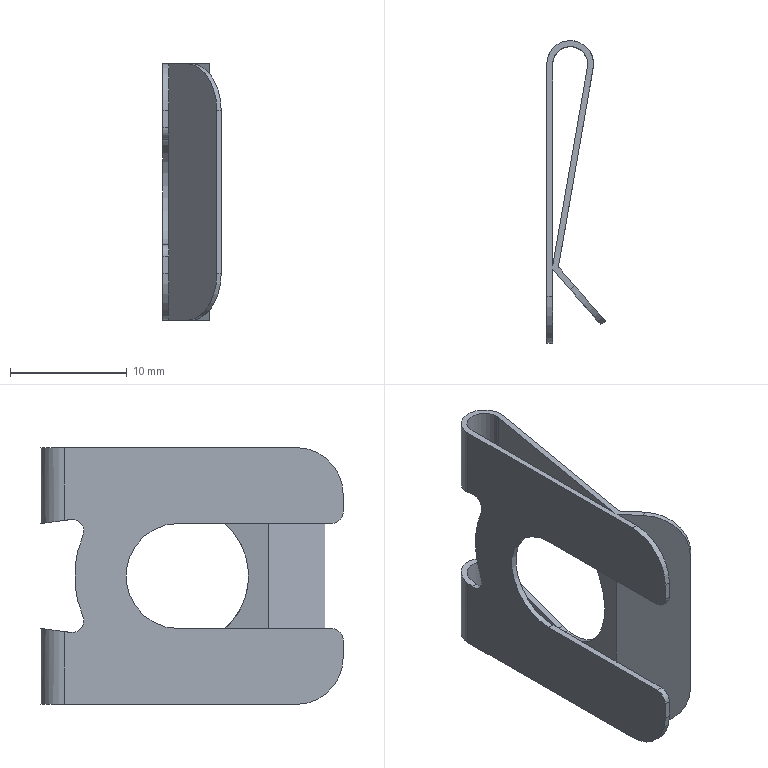Part | SolidWorks | features Fillet 3, ICE 2, BaseBody 1 | 1 solid | 40 faces | box 5 x 25.9 x 22 mm | volume 386.551 mm3 | cylinder 23 | plane 17 | commonest cylinder face diameters 2 x5 3 x4 4 x4 8 x4 12 x3 0.5 x1
STEP:
#1=CARTESIAN_POINT('',(0.5,9.8,-11.));
#2=VERTEX_POINT('',#1);
#3=CARTESIAN_POINT('',(3.5,9.8,-11.));
#4=VERTEX_POINT('',#3);
#5=CARTESIAN_POINT('',(2.,9.8,-11.));
#6=DIRECTION('',(0.,0.,-1.));
#7=DIRECTION('',(1.,0.,0.));
#8=AXIS2_PLACEMENT_3D('',#5,#6,#7);
#9=CIRCLE('',#8,1.5);
#10=EDGE_CURVE('',#2,#4,#9,.T.);
#11=ORIENTED_EDGE('',*,*,#10,.T.);
#12=CARTESIAN_POINT('',(3.5,9.8,-4.763));
#13=VERTEX_POINT('',#12);
#14=CARTESIAN_POINT('',(3.5,9.8,11.));
#15=DIRECTION('',(0.,0.,1.));
#16=VECTOR('',#15,1000.);
#17=LINE('',#14,#16);
#18=EDGE_CURVE('',#4,#13,#17,.T.);
#19=ORIENTED_EDGE('',*,*,#18,.T.);
#20=CARTESIAN_POINT('',(0.5,9.8,-4.763));
#21=VERTEX_POINT('',#20);
#22=CARTESIAN_POINT('',(0.5,9.8,-4.763));
#23=CARTESIAN_POINT('',(0.5,12.8,-4.369));
#24=CARTESIAN_POINT('',(3.5,12.8,-4.369));
#25=CARTESIAN_POINT('',(3.5,9.8,-4.763));
#26=(BOUNDED_CURVE()B_SPLINE_CURVE(3,(#22,#23,#24,#25),.UNSPECIFIED.,.F.,.F.)B_SPLINE_CURVE_WITH_KNOTS((4,4),(4.712,7.854),.UNSPECIFIED.)CURVE()GEOMETRIC_REPRESENTATION_ITEM()RATIONAL_B_SPLINE_CURVE((1.,0.3333,0.3333,1.))REPRESENTATION_ITEM(''));
#27=EDGE_CURVE('',#21,#13,#26,.T.);
#28=ORIENTED_EDGE('',*,*,#27,.F.);
#29=CARTESIAN_POINT('',(0.5,9.8,11.));
#30=DIRECTION('',(0.,0.,-1.));
#31=VECTOR('',#30,1000.);
#32=LINE('',#29,#31);
#33=EDGE_CURVE('',#21,#2,#32,.T.);
#34=ORIENTED_EDGE('',*,*,#33,.T.);
#35=EDGE_LOOP('',(#11,#19,#28,#34));
#36=FACE_OUTER_BOUND('',#35,.T.);
#37=CARTESIAN_POINT('',(2.,9.8,11.));
#38=DIRECTION('',(0.,0.,1.));
#39=DIRECTION('',(1.,0.,0.));
#40=AXIS2_PLACEMENT_3D('',#37,#38,#39);
#41=CYLINDRICAL_SURFACE('',#40,1.5);
#42=ADVANCED_FACE('',(#36),#41,.F.);
#43=CARTESIAN_POINT('',(0.5,9.254,4.835));
#44=VERTEX_POINT('',#43);
#45=CARTESIAN_POINT('',(0.5,9.124,4.843));
#46=VERTEX_POINT('',#45);
#47=CARTESIAN_POINT('',(0.5,9.124,3.843));
#48=DIRECTION('',(1.,0.,0.));
#49=DIRECTION('',(0.,0.,1.));
#50=AXIS2_PLACEMENT_3D('',#47,#48,#49);
#51=CIRCLE('',#50,1.);
#52=EDGE_CURVE('',#44,#46,#51,.T.);
#53=ORIENTED_EDGE('',*,*,#52,.T.);
#54=CARTESIAN_POINT('',(0.,9.124,4.843));
#55=VERTEX_POINT('',#54);
#56=CARTESIAN_POINT('',(-4.5,9.124,4.843));
#57=DIRECTION('',(-1.,0.,0.));
#58=VECTOR('',#57,1000.);
#59=LINE('',#56,#58);
#60=EDGE_CURVE('',#46,#55,#59,.T.);
#61=ORIENTED_EDGE('',*,*,#60,.T.);
#62=CARTESIAN_POINT('',(0.,9.254,4.835));
#63=VERTEX_POINT('',#62);
#64=CARTESIAN_POINT('',(0.,9.124,3.843));
#65=DIRECTION('',(1.,0.,0.));
#66=DIRECTION('',(0.,0.,1.));
#67=AXIS2_PLACEMENT_3D('',#64,#65,#66);
#68=CIRCLE('',#67,1.);
#69=EDGE_CURVE('',#63,#55,#68,.T.);
#70=ORIENTED_EDGE('',*,*,#69,.F.);
#71=CARTESIAN_POINT('',(5.5,9.254,4.835));
#72=DIRECTION('',(-1.,0.,0.));
#73=VECTOR('',#72,1000.);
#74=LINE('',#71,#73);
#75=EDGE_CURVE('',#44,#63,#74,.T.);
#76=ORIENTED_EDGE('',*,*,#75,.F.);
#77=EDGE_LOOP('',(#53,#61,#70,#76));
#78=FACE_OUTER_BOUND('',#77,.T.);
#79=CARTESIAN_POINT('',(-4.5,9.124,3.843));
#80=DIRECTION('',(-1.,0.,0.));
#81=DIRECTION('',(0.,0.,1.));
#82=AXIS2_PLACEMENT_3D('',#79,#80,#81);
#83=CYLINDRICAL_SURFACE('',#82,1.);
#84=ADVANCED_FACE('',(#78),#83,.F.);
#85=CARTESIAN_POINT('',(3.5,9.8,4.763));
#86=VERTEX_POINT('',#85);
#87=CARTESIAN_POINT('',(0.5,9.8,4.763));
#88=VERTEX_POINT('',#87);
#89=CARTESIAN_POINT('',(3.5,9.8,4.763));
#90=CARTESIAN_POINT('',(3.5,12.8,4.369));
#91=CARTESIAN_POINT('',(0.5,12.8,4.369));
#92=CARTESIAN_POINT('',(0.5,9.8,4.763));
#93=(BOUNDED_CURVE()B_SPLINE_CURVE(3,(#89,#90,#91,#92),.UNSPECIFIED.,.F.,.F.)B_SPLINE_CURVE_WITH_KNOTS((4,4),(1.571,4.712),.UNSPECIFIED.)CURVE()GEOMETRIC_REPRESENTATION_ITEM()RATIONAL_B_SPLINE_CURVE((1.,0.3333,0.3333,1.))REPRESENTATION_ITEM(''));
#94=EDGE_CURVE('',#86,#88,#93,.T.);
#95=ORIENTED_EDGE('',*,*,#94,.F.);
#96=CARTESIAN_POINT('',(3.5,9.8,11.));
#97=VERTEX_POINT('',#96);
#98=CARTESIAN_POINT('',(3.5,9.8,11.));
#99=DIRECTION('',(0.,0.,1.));
#100=VECTOR('',#99,1000.);
#101=LINE('',#98,#100);
#102=EDGE_CURVE('',#86,#97,#101,.T.);
#103=ORIENTED_EDGE('',*,*,#102,.T.);
#104=CARTESIAN_POINT('',(0.5,9.8,11.));
#105=VERTEX_POINT('',#104);
#106=CARTESIAN_POINT('',(2.,9.8,11.));
#107=DIRECTION('',(0.,0.,-1.));
#108=DIRECTION('',(1.,0.,0.));
#109=AXIS2_PLACEMENT_3D('',#106,#107,#108);
#110=CIRCLE('',#109,1.5);
#111=EDGE_CURVE('',#105,#97,#110,.T.);
#112=ORIENTED_EDGE('',*,*,#111,.F.);
#113=CARTESIAN_POINT('',(0.5,9.8,11.));
#114=DIRECTION('',(0.,0.,-1.));
#115=VECTOR('',#114,1000.);
#116=LINE('',#113,#115);
#117=EDGE_CURVE('',#105,#88,#116,.T.);
#118=ORIENTED_EDGE('',*,*,#117,.T.);
#119=EDGE_LOOP('',(#95,#103,#112,#118));
#120=FACE_OUTER_BOUND('',#119,.T.);
#121=CARTESIAN_POINT('',(2.,9.8,11.));
#122=DIRECTION('',(0.,0.,1.));
#123=DIRECTION('',(1.,0.,0.));
#124=AXIS2_PLACEMENT_3D('',#121,#122,#123);
#125=CYLINDRICAL_SURFACE('',#124,1.5);
#126=ADVANCED_FACE('',(#120),#125,.F.);
#127=CARTESIAN_POINT('',(3.97,9.456,-11.));
#128=VERTEX_POINT('',#127);
#129=CARTESIAN_POINT('',(4.,9.8,-11.));
#130=VERTEX_POINT('',#129);
#131=CARTESIAN_POINT('',(2.,9.8,-11.));
#132=DIRECTION('',(0.,0.,1.));
#133=DIRECTION('',(1.,0.,0.));
#134=AXIS2_PLACEMENT_3D('',#131,#132,#133);
#135=CIRCLE('',#134,2.);
#136=EDGE_CURVE('',#128,#130,#135,.T.);
#137=ORIENTED_EDGE('',*,*,#136,.T.);
#138=CARTESIAN_POINT('',(4.,9.8,-4.763));
#139=VERTEX_POINT('',#138);
#140=CARTESIAN_POINT('',(4.,9.8,11.));
#141=DIRECTION('',(0.,0.,1.));
#142=VECTOR('',#141,1000.);
#143=LINE('',#140,#142);
#144=EDGE_CURVE('',#130,#139,#143,.T.);
#145=ORIENTED_EDGE('',*,*,#144,.T.);
#146=CARTESIAN_POINT('',(3.97,9.456,-4.808));
#147=VERTEX_POINT('',#146);
#148=CARTESIAN_POINT('',(4.,9.8,-4.763));
#149=CARTESIAN_POINT('',(4.,9.685,-4.778));
#150=CARTESIAN_POINT('',(3.99,9.57,-4.793));
#151=CARTESIAN_POINT('',(3.97,9.456,-4.808));
#152=(BOUNDED_CURVE()B_SPLINE_CURVE(3,(#148,#149,#150,#151),.UNSPECIFIED.,.F.,.F.)B_SPLINE_CURVE_WITH_KNOTS((4,4),(1.571,1.744),.UNSPECIFIED.)CURVE()GEOMETRIC_REPRESENTATION_ITEM()RATIONAL_B_SPLINE_CURVE((1.,0.9975,0.9975,1.))REPRESENTATION_ITEM(''));
#153=EDGE_CURVE('',#139,#147,#152,.T.);
#154=ORIENTED_EDGE('',*,*,#153,.T.);
#155=CARTESIAN_POINT('',(3.97,9.456,11.));
#156=DIRECTION('',(0.,0.,-1.));
#157=VECTOR('',#156,1000.);
#158=LINE('',#155,#157);
#159=EDGE_CURVE('',#147,#128,#158,.T.);
#160=ORIENTED_EDGE('',*,*,#159,.T.);
#161=EDGE_LOOP('',(#137,#145,#154,#160));
#162=FACE_OUTER_BOUND('',#161,.T.);
#163=CARTESIAN_POINT('',(2.,9.8,11.));
#164=DIRECTION('',(0.,0.,1.));
#165=DIRECTION('',(1.,0.,0.));
#166=AXIS2_PLACEMENT_3D('',#163,#164,#165);
#167=CYLINDRICAL_SURFACE('',#166,2.);
#168=ADVANCED_FACE('',(#162),#167,.T.);
#169=CARTESIAN_POINT('',(4.,9.8,4.763));
#170=VERTEX_POINT('',#169);
#171=CARTESIAN_POINT('',(3.97,9.456,4.808));
#172=VERTEX_POINT('',#171);
#173=CARTESIAN_POINT('',(4.,9.8,4.763));
#174=CARTESIAN_POINT('',(4.,9.685,4.778));
#175=CARTESIAN_POINT('',(3.99,9.57,4.793));
#176=CARTESIAN_POINT('',(3.97,9.456,4.808));
#177=(BOUNDED_CURVE()B_SPLINE_CURVE(3,(#173,#174,#175,#176),.UNSPECIFIED.,.F.,.F.)B_SPLINE_CURVE_WITH_KNOTS((4,4),(4.712,4.885),.UNSPECIFIED.)CURVE()GEOMETRIC_REPRESENTATION_ITEM()RATIONAL_B_SPLINE_CURVE((1.,0.9975,0.9975,1.))REPRESENTATION_ITEM(''));
#178=EDGE_CURVE('',#170,#172,#177,.T.);
#179=ORIENTED_EDGE('',*,*,#178,.F.);
#180=CARTESIAN_POINT('',(4.,9.8,11.));
#181=VERTEX_POINT('',#180);
#182=CARTESIAN_POINT('',(4.,9.8,11.));
#183=DIRECTION('',(0.,0.,1.));
#184=VECTOR('',#183,1000.);
#185=LINE('',#182,#184);
#186=EDGE_CURVE('',#170,#181,#185,.T.);
#187=ORIENTED_EDGE('',*,*,#186,.T.);
#188=CARTESIAN_POINT('',(3.97,9.456,11.));
#189=VERTEX_POINT('',#188);
#190=CARTESIAN_POINT('',(2.,9.8,11.));
#191=DIRECTION('',(0.,0.,1.));
#192=DIRECTION('',(1.,0.,0.));
#193=AXIS2_PLACEMENT_3D('',#190,#191,#192);
#194=CIRCLE('',#193,2.);
#195=EDGE_CURVE('',#189,#181,#194,.T.);
#196=ORIENTED_EDGE('',*,*,#195,.F.);
#197=CARTESIAN_POINT('',(3.97,9.456,11.));
#198=DIRECTION('',(0.,0.,-1.));
#199=VECTOR('',#198,1000.);
#200=LINE('',#197,#199);
#201=EDGE_CURVE('',#189,#172,#200,.T.);
#202=ORIENTED_EDGE('',*,*,#201,.T.);
#203=EDGE_LOOP('',(#179,#187,#196,#202));
#204=FACE_OUTER_BOUND('',#203,.T.);
#205=CARTESIAN_POINT('',(2.,9.8,11.));
#206=DIRECTION('',(0.,0.,1.));
#207=DIRECTION('',(1.,0.,0.));
#208=AXIS2_PLACEMENT_3D('',#205,#206,#207);
#209=CYLINDRICAL_SURFACE('',#208,2.);
#210=ADVANCED_FACE('',(#204),#209,.T.);
#211=CARTESIAN_POINT('',(1.81,0.,-6.));
#212=VERTEX_POINT('',#211);
#213=CARTESIAN_POINT('',(1.81,0.,6.));
#214=VERTEX_POINT('',#213);
#215=CARTESIAN_POINT('',(1.81,0.,-6.));
#216=CARTESIAN_POINT('',(-0.2863,-12.,-6.));
#217=CARTESIAN_POINT('',(-0.2863,-12.,6.));
#218=CARTESIAN_POINT('',(1.81,0.,6.));
#219=(BOUNDED_CURVE()B_SPLINE_CURVE(3,(#215,#216,#217,#218),.UNSPECIFIED.,.F.,.F.)B_SPLINE_CURVE_WITH_KNOTS((4,4),(1.571,4.712),.UNSPECIFIED.)CURVE()GEOMETRIC_REPRESENTATION_ITEM()RATIONAL_B_SPLINE_CURVE((1.,0.3333,0.3333,1.))REPRESENTATION_ITEM(''));
#220=EDGE_CURVE('',#212,#214,#219,.T.);
#221=ORIENTED_EDGE('',*,*,#220,.T.);
#222=CARTESIAN_POINT('',(2.318,0.,6.));
#223=VERTEX_POINT('',#222);
#224=CARTESIAN_POINT('',(5.5,0.,6.));
#225=DIRECTION('',(1.,0.,0.));
#226=VECTOR('',#225,1000.);
#227=LINE('',#224,#226);
#228=EDGE_CURVE('',#214,#223,#227,.T.);
#229=ORIENTED_EDGE('',*,*,#228,.T.);
#230=CARTESIAN_POINT('',(2.318,0.,-6.));
#231=VERTEX_POINT('',#230);
#232=CARTESIAN_POINT('',(2.318,0.,6.));
#233=CARTESIAN_POINT('',(0.2213,-12.,6.));
#234=CARTESIAN_POINT('',(0.2213,-12.,-6.));
#235=CARTESIAN_POINT('',(2.318,0.,-6.));
#236=(BOUNDED_CURVE()B_SPLINE_CURVE(3,(#232,#233,#234,#235),.UNSPECIFIED.,.F.,.T.)B_SPLINE_CURVE_WITH_KNOTS((4,4),(1.571,4.712),.UNSPECIFIED.)CURVE()GEOMETRIC_REPRESENTATION_ITEM()RATIONAL_B_SPLINE_CURVE((1.,0.3333,0.3333,1.))REPRESENTATION_ITEM(''));
#237=EDGE_CURVE('',#223,#231,#236,.T.);
#238=ORIENTED_EDGE('',*,*,#237,.T.);
#239=CARTESIAN_POINT('',(5.5,0.,-6.));
#240=DIRECTION('',(1.,0.,0.));
#241=VECTOR('',#240,1000.);
#242=LINE('',#239,#241);
#243=EDGE_CURVE('',#212,#231,#242,.T.);
#244=ORIENTED_EDGE('',*,*,#243,.F.);
#245=EDGE_LOOP('',(#221,#229,#238,#244));
#246=FACE_OUTER_BOUND('',#245,.T.);
#247=CARTESIAN_POINT('',(5.5,0.,0.));
#248=DIRECTION('',(1.,0.,0.));
#249=DIRECTION('',(0.,0.,-1.));
#250=AXIS2_PLACEMENT_3D('',#247,#248,#249);
#251=CYLINDRICAL_SURFACE('',#250,6.);
#252=ADVANCED_FACE('',(#246),#251,.F.);
#253=CARTESIAN_POINT('',(1.947,0.7822,-5.949));
#254=VERTEX_POINT('',#253);
#255=CARTESIAN_POINT('',(1.947,0.7822,-5.949));
#256=CARTESIAN_POINT('',(1.902,0.5228,-5.983));
#257=CARTESIAN_POINT('',(1.856,0.2617,-6.));
#258=CARTESIAN_POINT('',(1.81,0.,-6.));
#259=(BOUNDED_CURVE()B_SPLINE_CURVE(3,(#255,#256,#257,#258),.UNSPECIFIED.,.F.,.F.)B_SPLINE_CURVE_WITH_KNOTS((4,4),(1.44,1.571),.UNSPECIFIED.)CURVE()GEOMETRIC_REPRESENTATION_ITEM()RATIONAL_B_SPLINE_CURVE((1.,0.9986,0.9986,1.))REPRESENTATION_ITEM(''));
#260=EDGE_CURVE('',#254,#212,#259,.T.);
#261=ORIENTED_EDGE('',*,*,#260,.T.);
#262=ORIENTED_EDGE('',*,*,#243,.T.);
#263=CARTESIAN_POINT('',(2.455,0.7822,-5.949));
#264=VERTEX_POINT('',#263);
#265=CARTESIAN_POINT('',(2.318,0.,-6.));
#266=CARTESIAN_POINT('',(2.364,0.2617,-6.));
#267=CARTESIAN_POINT('',(2.409,0.5228,-5.983));
#268=CARTESIAN_POINT('',(2.455,0.7822,-5.949));
#269=(BOUNDED_CURVE()B_SPLINE_CURVE(3,(#265,#266,#267,#268),.UNSPECIFIED.,.F.,.F.)B_SPLINE_CURVE_WITH_KNOTS((4,4),(4.712,4.843),.UNSPECIFIED.)CURVE()GEOMETRIC_REPRESENTATION_ITEM()RATIONAL_B_SPLINE_CURVE((1.,0.9986,0.9986,1.))REPRESENTATION_ITEM(''));
#270=EDGE_CURVE('',#231,#264,#269,.T.);
#271=ORIENTED_EDGE('',*,*,#270,.T.);
#272=CARTESIAN_POINT('',(5.5,0.7822,-5.949));
#273=DIRECTION('',(1.,0.,0.));
#274=VECTOR('',#273,1000.);
#275=LINE('',#272,#274);
#276=EDGE_CURVE('',#254,#264,#275,.T.);
#277=ORIENTED_EDGE('',*,*,#276,.F.);
#278=EDGE_LOOP('',(#261,#262,#271,#277));
#279=FACE_OUTER_BOUND('',#278,.T.);
#280=CARTESIAN_POINT('',(5.5,0.,0.));
#281=DIRECTION('',(1.,0.,0.));
#282=DIRECTION('',(0.,0.,-1.));
#283=AXIS2_PLACEMENT_3D('',#280,#281,#282);
#284=CYLINDRICAL_SURFACE('',#283,6.);
#285=ADVANCED_FACE('',(#279),#284,.F.);
#286=CARTESIAN_POINT('',(0.4591,-7.734,-4.5));
#287=VERTEX_POINT('',#286);
#288=CARTESIAN_POINT('',(0.5,-7.5,-4.5));
#289=VERTEX_POINT('',#288);
#290=CARTESIAN_POINT('',(-0.619,-13.904,-4.5));
#291=DIRECTION('',(0.1721,0.9851,0.));
#292=VECTOR('',#291,1000.);
#293=LINE('',#290,#292);
#294=EDGE_CURVE('',#287,#289,#293,.T.);
#295=ORIENTED_EDGE('',*,*,#294,.F.);
#296=CARTESIAN_POINT('',(0.4591,-7.734,4.5));
#297=VERTEX_POINT('',#296);
#298=CARTESIAN_POINT('',(0.4591,-7.734,11.));
#299=DIRECTION('',(0.,0.,-1.));
#300=VECTOR('',#299,1000.);
#301=LINE('',#298,#300);
#302=EDGE_CURVE('',#297,#287,#301,.T.);
#303=ORIENTED_EDGE('',*,*,#302,.F.);
#304=CARTESIAN_POINT('',(0.5,-7.5,4.5));
#305=VERTEX_POINT('',#304);
#306=CARTESIAN_POINT('',(1.772,-0.2222,4.5));
#307=DIRECTION('',(-0.1721,-0.9851,0.));
#308=VECTOR('',#307,1000.);
#309=LINE('',#306,#308);
#310=EDGE_CURVE('',#305,#297,#309,.T.);
#311=ORIENTED_EDGE('',*,*,#310,.F.);
#312=CARTESIAN_POINT('',(0.5,-7.5,11.));
#313=VERTEX_POINT('',#312);
#314=CARTESIAN_POINT('',(0.5,-7.5,11.));
#315=DIRECTION('',(0.,0.,1.));
#316=VECTOR('',#315,1000.);
#317=LINE('',#314,#316);
#318=EDGE_CURVE('',#305,#313,#317,.T.);
#319=ORIENTED_EDGE('',*,*,#318,.T.);
#320=CARTESIAN_POINT('',(3.478,9.542,11.));
#321=VERTEX_POINT('',#320);
#322=CARTESIAN_POINT('',(3.478,9.542,11.));
#323=DIRECTION('',(-0.1721,-0.9851,0.));
#324=VECTOR('',#323,1000.);
#325=LINE('',#322,#324);
#326=EDGE_CURVE('',#321,#313,#325,.T.);
#327=ORIENTED_EDGE('',*,*,#326,.F.);
#328=CARTESIAN_POINT('',(3.478,9.542,4.797));
#329=VERTEX_POINT('',#328);
#330=CARTESIAN_POINT('',(3.478,9.542,11.));
#331=DIRECTION('',(0.,0.,1.));
#332=VECTOR('',#331,1000.);
#333=LINE('',#330,#332);
#334=EDGE_CURVE('',#329,#321,#333,.T.);
#335=ORIENTED_EDGE('',*,*,#334,.F.);
#336=CARTESIAN_POINT('',(1.947,0.7822,5.949));
#337=VERTEX_POINT('',#336);
#338=CARTESIAN_POINT('',(1.947,0.7822,5.949));
#339=DIRECTION('',(0.1707,0.9769,-0.1285));
#340=VECTOR('',#339,1000.);
#341=LINE('',#338,#340);
#342=EDGE_CURVE('',#337,#329,#341,.T.);
#343=ORIENTED_EDGE('',*,*,#342,.F.);
#344=CARTESIAN_POINT('',(1.81,0.,6.));
#345=CARTESIAN_POINT('',(1.856,0.2617,6.));
#346=CARTESIAN_POINT('',(1.902,0.5228,5.983));
#347=CARTESIAN_POINT('',(1.947,0.7822,5.949));
#348=(BOUNDED_CURVE()B_SPLINE_CURVE(3,(#344,#345,#346,#347),.UNSPECIFIED.,.F.,.F.)B_SPLINE_CURVE_WITH_KNOTS((4,4),(4.712,4.843),.UNSPECIFIED.)CURVE()GEOMETRIC_REPRESENTATION_ITEM()RATIONAL_B_SPLINE_CURVE((1.,0.9986,0.9986,1.))REPRESENTATION_ITEM(''));
#349=EDGE_CURVE('',#214,#337,#348,.T.);
#350=ORIENTED_EDGE('',*,*,#349,.F.);
#351=ORIENTED_EDGE('',*,*,#220,.F.);
#352=ORIENTED_EDGE('',*,*,#260,.F.);
#353=CARTESIAN_POINT('',(3.478,9.542,-4.797));
#354=VERTEX_POINT('',#353);
#355=CARTESIAN_POINT('',(3.478,9.542,-4.797));
#356=DIRECTION('',(-0.1707,-0.9769,-0.1285));
#357=VECTOR('',#356,1000.);
#358=LINE('',#355,#357);
#359=EDGE_CURVE('',#354,#254,#358,.T.);
#360=ORIENTED_EDGE('',*,*,#359,.F.);
#361=CARTESIAN_POINT('',(3.478,9.542,-11.));
#362=VERTEX_POINT('',#361);
#363=CARTESIAN_POINT('',(3.478,9.542,11.));
#364=DIRECTION('',(0.,0.,1.));
#365=VECTOR('',#364,1000.);
#366=LINE('',#363,#365);
#367=EDGE_CURVE('',#362,#354,#366,.T.);
#368=ORIENTED_EDGE('',*,*,#367,.F.);
#369=CARTESIAN_POINT('',(0.5,-7.5,-11.));
#370=VERTEX_POINT('',#369);
#371=CARTESIAN_POINT('',(3.478,9.542,-11.));
#372=DIRECTION('',(-0.1721,-0.9851,0.));
#373=VECTOR('',#372,1000.);
#374=LINE('',#371,#373);
#375=EDGE_CURVE('',#362,#370,#374,.T.);
#376=ORIENTED_EDGE('',*,*,#375,.T.);
#377=CARTESIAN_POINT('',(0.5,-7.5,11.));
#378=DIRECTION('',(0.,0.,1.));
#379=VECTOR('',#378,1000.);
#380=LINE('',#377,#379);
#381=EDGE_CURVE('',#370,#289,#380,.T.);
#382=ORIENTED_EDGE('',*,*,#381,.T.);
#383=EDGE_LOOP('',(#295,#303,#311,#319,#327,#335,#343,#350,#351,#352,#360,#368,#376,#382));
#384=FACE_OUTER_BOUND('',#383,.T.);
#385=CARTESIAN_POINT('',(3.478,9.542,11.));
#386=DIRECTION('',(0.9851,-0.1721,0.));
#387=DIRECTION('',(0.,0.,-1.));
#388=AXIS2_PLACEMENT_3D('',#385,#386,#387);
#389=PLANE('',#388);
#390=ADVANCED_FACE('',(#384),#389,.F.);
#391=ORIENTED_EDGE('',*,*,#381,.F.);
#392=CARTESIAN_POINT('',(0.5,-14.1,-11.));
#393=DIRECTION('',(0.,-1.,0.));
#394=VECTOR('',#393,1000.);
#395=LINE('',#392,#394);
#396=EDGE_CURVE('',#2,#370,#395,.T.);
#397=ORIENTED_EDGE('',*,*,#396,.F.);
#398=ORIENTED_EDGE('',*,*,#33,.F.);
#399=CARTESIAN_POINT('',(0.5,9.254,-4.835));
#400=VERTEX_POINT('',#399);
#401=CARTESIAN_POINT('',(0.5,0.7822,-5.949));
#402=DIRECTION('',(0.,0.9915,0.1304));
#403=VECTOR('',#402,1000.);
#404=LINE('',#401,#403);
#405=EDGE_CURVE('',#400,#21,#404,.T.);
#406=ORIENTED_EDGE('',*,*,#405,.F.);
#407=CARTESIAN_POINT('',(0.5,8.202,-3.455));
#408=VERTEX_POINT('',#407);
#409=CARTESIAN_POINT('',(0.5,9.124,-3.843));
#410=DIRECTION('',(1.,0.,0.));
#411=DIRECTION('',(0.,0.,1.));
#412=AXIS2_PLACEMENT_3D('',#409,#410,#411);
#413=CIRCLE('',#412,1.);
#414=EDGE_CURVE('',#408,#400,#413,.T.);
#415=ORIENTED_EDGE('',*,*,#414,.F.);
#416=CARTESIAN_POINT('',(0.5,8.202,3.455));
#417=VERTEX_POINT('',#416);
#418=CARTESIAN_POINT('',(0.5,0.,0.));
#419=DIRECTION('',(-1.,0.,0.));
#420=DIRECTION('',(0.,0.,1.));
#421=AXIS2_PLACEMENT_3D('',#418,#419,#420);
#422=CIRCLE('',#421,8.9);
#423=EDGE_CURVE('',#417,#408,#422,.T.);
#424=ORIENTED_EDGE('',*,*,#423,.F.);
#425=CARTESIAN_POINT('',(0.5,9.124,3.843));
#426=DIRECTION('',(1.,0.,0.));
#427=DIRECTION('',(0.,0.,1.));
#428=AXIS2_PLACEMENT_3D('',#425,#426,#427);
#429=CIRCLE('',#428,1.);
#430=EDGE_CURVE('',#46,#417,#429,.T.);
#431=ORIENTED_EDGE('',*,*,#430,.F.);
#432=ORIENTED_EDGE('',*,*,#52,.F.);
#433=CARTESIAN_POINT('',(0.5,11.8,4.5));
#434=DIRECTION('',(0.,-0.9915,0.1304));
#435=VECTOR('',#434,1000.);
#436=LINE('',#433,#435);
#437=EDGE_CURVE('',#88,#44,#436,.T.);
#438=ORIENTED_EDGE('',*,*,#437,.F.);
#439=ORIENTED_EDGE('',*,*,#117,.F.);
#440=CARTESIAN_POINT('',(0.5,-14.1,11.));
#441=DIRECTION('',(0.,1.,0.));
#442=VECTOR('',#441,1000.);
#443=LINE('',#440,#442);
#444=EDGE_CURVE('',#313,#105,#443,.T.);
#445=ORIENTED_EDGE('',*,*,#444,.F.);
#446=ORIENTED_EDGE('',*,*,#318,.F.);
#447=CARTESIAN_POINT('',(0.5,0.,4.5));
#448=VERTEX_POINT('',#447);
#449=CARTESIAN_POINT('',(0.5,-14.1,4.5));
#450=DIRECTION('',(0.,-1.,0.));
#451=VECTOR('',#450,1000.);
#452=LINE('',#449,#451);
#453=EDGE_CURVE('',#448,#305,#452,.T.);
#454=ORIENTED_EDGE('',*,*,#453,.F.);
#455=CARTESIAN_POINT('',(0.5,0.,-4.5));
#456=VERTEX_POINT('',#455);
#457=CARTESIAN_POINT('',(0.5,0.,0.));
#458=DIRECTION('',(1.,0.,0.));
#459=DIRECTION('',(0.,0.,-1.));
#460=AXIS2_PLACEMENT_3D('',#457,#458,#459);
#461=CIRCLE('',#460,4.5);
#462=EDGE_CURVE('',#456,#448,#461,.T.);
#463=ORIENTED_EDGE('',*,*,#462,.F.);
#464=CARTESIAN_POINT('',(0.5,-14.1,-4.5));
#465=DIRECTION('',(0.,1.,0.));
#466=VECTOR('',#465,1000.);
#467=LINE('',#464,#466);
#468=EDGE_CURVE('',#289,#456,#467,.T.);
#469=ORIENTED_EDGE('',*,*,#468,.F.);
#470=EDGE_LOOP('',(#391,#397,#398,#406,#415,#424,#431,#432,#438,#439,#445,#446,#454,#463,#469));
#471=FACE_OUTER_BOUND('',#470,.T.);
#472=CARTESIAN_POINT('',(0.5,-14.1,11.));
#473=DIRECTION('',(-1.,0.,0.));
#474=DIRECTION('',(0.,0.,1.));
#475=AXIS2_PLACEMENT_3D('',#472,#473,#474);
#476=PLANE('',#475);
#477=ADVANCED_FACE('',(#471),#476,.F.);
#478=CARTESIAN_POINT('',(4.622,-12.528,7.));
#479=VERTEX_POINT('',#478);
#480=CARTESIAN_POINT('',(4.622,-12.528,-7.));
#481=VERTEX_POINT('',#480);
#482=CARTESIAN_POINT('',(4.622,-12.528,11.));
#483=DIRECTION('',(0.,0.,-1.));
#484=VECTOR('',#483,1000.);
#485=LINE('',#482,#484);
#486=EDGE_CURVE('',#479,#481,#485,.T.);
#487=ORIENTED_EDGE('',*,*,#486,.T.);
#488=CARTESIAN_POINT('',(5.,-12.2,-7.));
#489=VERTEX_POINT('',#488);
#490=CARTESIAN_POINT('',(5.,-12.2,-7.));
#491=DIRECTION('',(0.755,0.6557,0.));
#492=VECTOR('',#491,1000.);
#493=LINE('',#490,#492);
#494=EDGE_CURVE('',#481,#489,#493,.T.);
#495=ORIENTED_EDGE('',*,*,#494,.T.);
#496=CARTESIAN_POINT('',(5.,-12.2,7.));
#497=VERTEX_POINT('',#496);
#498=CARTESIAN_POINT('',(5.,-12.2,11.));
#499=DIRECTION('',(0.,0.,1.));
#500=VECTOR('',#499,1000.);
#501=LINE('',#498,#500);
#502=EDGE_CURVE('',#489,#497,#501,.T.);
#503=ORIENTED_EDGE('',*,*,#502,.T.);
#504=CARTESIAN_POINT('',(5.755,-11.544,7.));
#505=DIRECTION('',(-0.755,-0.6557,0.));
#506=VECTOR('',#505,1000.);
#507=LINE('',#504,#506);
#508=EDGE_CURVE('',#497,#479,#507,.T.);
#509=ORIENTED_EDGE('',*,*,#508,.T.);
#510=EDGE_LOOP('',(#487,#495,#503,#509));
#511=FACE_OUTER_BOUND('',#510,.T.);
#512=CARTESIAN_POINT('',(5.755,-11.544,-7.));
#513=DIRECTION('',(0.6557,-0.755,0.));
#514=DIRECTION('',(0.,0.,-1.));
#515=AXIS2_PLACEMENT_3D('',#512,#513,#514);
#516=PLANE('',#515);
#517=ADVANCED_FACE('',(#511),#516,.T.);
#518=CARTESIAN_POINT('',(0.,9.8,4.763));
#519=VERTEX_POINT('',#518);
#520=CARTESIAN_POINT('',(0.,9.8,4.763));
#521=CARTESIAN_POINT('',(0.,13.8,4.237));
#522=CARTESIAN_POINT('',(4.,13.8,4.237));
#523=CARTESIAN_POINT('',(4.,9.8,4.763));
#524=(BOUNDED_CURVE()B_SPLINE_CURVE(3,(#520,#521,#522,#523),.UNSPECIFIED.,.F.,.T.)B_SPLINE_CURVE_WITH_KNOTS((4,4),(1.571,4.712),.UNSPECIFIED.)CURVE()GEOMETRIC_REPRESENTATION_ITEM()RATIONAL_B_SPLINE_CURVE((1.,0.3333,0.3333,1.))REPRESENTATION_ITEM(''));
#525=EDGE_CURVE('',#519,#170,#524,.T.);
#526=ORIENTED_EDGE('',*,*,#525,.T.);
#527=ORIENTED_EDGE('',*,*,#178,.T.);
#528=CARTESIAN_POINT('',(2.455,0.7822,5.949));
#529=VERTEX_POINT('',#528);
#530=CARTESIAN_POINT('',(3.97,9.456,4.808));
#531=DIRECTION('',(-0.1707,-0.9769,0.1285));
#532=VECTOR('',#531,1000.);
#533=LINE('',#530,#532);
#534=EDGE_CURVE('',#172,#529,#533,.T.);
#535=ORIENTED_EDGE('',*,*,#534,.T.);
#536=CARTESIAN_POINT('',(5.5,0.7822,5.949));
#537=DIRECTION('',(-1.,0.,0.));
#538=VECTOR('',#537,1000.);
#539=LINE('',#536,#538);
#540=EDGE_CURVE('',#529,#337,#539,.T.);
#541=ORIENTED_EDGE('',*,*,#540,.T.);
#542=ORIENTED_EDGE('',*,*,#342,.T.);
#543=CARTESIAN_POINT('',(3.478,9.542,4.797));
#544=CARTESIAN_POINT('',(3.493,9.627,4.786));
#545=CARTESIAN_POINT('',(3.5,9.713,4.774));
#546=CARTESIAN_POINT('',(3.5,9.8,4.763));
#547=(BOUNDED_CURVE()B_SPLINE_CURVE(3,(#543,#544,#545,#546),.UNSPECIFIED.,.F.,.F.)B_SPLINE_CURVE_WITH_KNOTS((4,4),(1.398,1.571),.UNSPECIFIED.)CURVE()GEOMETRIC_REPRESENTATION_ITEM()RATIONAL_B_SPLINE_CURVE((1.,0.9975,0.9975,1.))REPRESENTATION_ITEM(''));
#548=EDGE_CURVE('',#329,#86,#547,.T.);
#549=ORIENTED_EDGE('',*,*,#548,.T.);
#550=ORIENTED_EDGE('',*,*,#94,.T.);
#551=ORIENTED_EDGE('',*,*,#437,.T.);
#552=ORIENTED_EDGE('',*,*,#75,.T.);
#553=CARTESIAN_POINT('',(0.,9.254,4.835));
#554=DIRECTION('',(0.,0.9915,-0.1304));
#555=VECTOR('',#554,1000.);
#556=LINE('',#553,#555);
#557=EDGE_CURVE('',#63,#519,#556,.T.);
#558=ORIENTED_EDGE('',*,*,#557,.T.);
#559=EDGE_LOOP('',(#526,#527,#535,#541,#542,#549,#550,#551,#552,#558));
#560=FACE_OUTER_BOUND('',#559,.T.);
#561=CARTESIAN_POINT('',(5.5,11.8,4.5));
#562=DIRECTION('',(0.,-0.1304,-0.9915));
#563=DIRECTION('',(0.,-0.9915,0.1304));
#564=AXIS2_PLACEMENT_3D('',#561,#562,#563);
#565=PLANE('',#564);
#566=ADVANCED_FACE('',(#560),#565,.T.);
#567=CARTESIAN_POINT('',(0.,9.8,-4.763));
#568=VERTEX_POINT('',#567);
#569=CARTESIAN_POINT('',(0.,9.254,-4.835));
#570=VERTEX_POINT('',#569);
#571=CARTESIAN_POINT('',(0.,9.8,-4.763));
#572=DIRECTION('',(0.,-0.9915,-0.1304));
#573=VECTOR('',#572,1000.);
#574=LINE('',#571,#573);
#575=EDGE_CURVE('',#568,#570,#574,.T.);
#576=ORIENTED_EDGE('',*,*,#575,.T.);
#577=CARTESIAN_POINT('',(-4.5,9.254,-4.835));
#578=DIRECTION('',(1.,0.,0.));
#579=VECTOR('',#578,1000.);
#580=LINE('',#577,#579);
#581=EDGE_CURVE('',#570,#400,#580,.T.);
#582=ORIENTED_EDGE('',*,*,#581,.T.);
#583=ORIENTED_EDGE('',*,*,#405,.T.);
#584=ORIENTED_EDGE('',*,*,#27,.T.);
#585=CARTESIAN_POINT('',(3.5,9.8,-4.763));
#586=CARTESIAN_POINT('',(3.5,9.713,-4.774));
#587=CARTESIAN_POINT('',(3.493,9.627,-4.786));
#588=CARTESIAN_POINT('',(3.478,9.542,-4.797));
#589=(BOUNDED_CURVE()B_SPLINE_CURVE(3,(#585,#586,#587,#588),.UNSPECIFIED.,.F.,.F.)B_SPLINE_CURVE_WITH_KNOTS((4,4),(1.571,1.744),.UNSPECIFIED.)CURVE()GEOMETRIC_REPRESENTATION_ITEM()RATIONAL_B_SPLINE_CURVE((1.,0.9975,0.9975,1.))REPRESENTATION_ITEM(''));
#590=EDGE_CURVE('',#13,#354,#589,.T.);
#591=ORIENTED_EDGE('',*,*,#590,.T.);
#592=ORIENTED_EDGE('',*,*,#359,.T.);
#593=ORIENTED_EDGE('',*,*,#276,.T.);
#594=CARTESIAN_POINT('',(2.455,0.7822,-5.949));
#595=DIRECTION('',(0.1707,0.9769,0.1285));
#596=VECTOR('',#595,1000.);
#597=LINE('',#594,#596);
#598=EDGE_CURVE('',#264,#147,#597,.T.);
#599=ORIENTED_EDGE('',*,*,#598,.T.);
#600=ORIENTED_EDGE('',*,*,#153,.F.);
#601=CARTESIAN_POINT('',(0.,9.8,-4.763));
#602=CARTESIAN_POINT('',(0.,13.8,-4.237));
#603=CARTESIAN_POINT('',(4.,13.8,-4.237));
#604=CARTESIAN_POINT('',(4.,9.8,-4.763));
#605=(BOUNDED_CURVE()B_SPLINE_CURVE(3,(#601,#602,#603,#604),.UNSPECIFIED.,.F.,.F.)B_SPLINE_CURVE_WITH_KNOTS((4,4),(4.712,7.854),.UNSPECIFIED.)CURVE()GEOMETRIC_REPRESENTATION_ITEM()RATIONAL_B_SPLINE_CURVE((1.,0.3333,0.3333,1.))REPRESENTATION_ITEM(''));
#606=EDGE_CURVE('',#568,#139,#605,.T.);
#607=ORIENTED_EDGE('',*,*,#606,.F.);
#608=EDGE_LOOP('',(#576,#582,#583,#584,#591,#592,#593,#599,#600,#607));
#609=FACE_OUTER_BOUND('',#608,.T.);
#610=CARTESIAN_POINT('',(5.5,0.7822,-5.949));
#611=DIRECTION('',(0.,-0.1304,0.9915));
#612=DIRECTION('',(-1.,0.,0.));
#613=AXIS2_PLACEMENT_3D('',#610,#611,#612);
#614=PLANE('',#613);
#615=ADVANCED_FACE('',(#609),#614,.T.);
#616=ORIENTED_EDGE('',*,*,#502,.F.);
#617=CARTESIAN_POINT('',(2.377,-9.18,-11.));
#618=VERTEX_POINT('',#617);
#619=CARTESIAN_POINT('',(2.377,-9.18,-7.));
#620=DIRECTION('',(0.755,0.6557,0.));
#621=DIRECTION('',(0.6557,-0.755,0.));
#622=AXIS2_PLACEMENT_3D('',#619,#620,#621);
#623=CIRCLE('',#622,4.);
#624=EDGE_CURVE('',#489,#618,#623,.T.);
#625=ORIENTED_EDGE('',*,*,#624,.T.);
#626=CARTESIAN_POINT('',(1.071,-7.676,-11.));
#627=VERTEX_POINT('',#626);
#628=CARTESIAN_POINT('',(2.377,-9.18,-11.));
#629=DIRECTION('',(-0.6557,0.755,0.));
#630=VECTOR('',#629,1000.);
#631=LINE('',#628,#630);
#632=EDGE_CURVE('',#618,#627,#631,.T.);
#633=ORIENTED_EDGE('',*,*,#632,.T.);
#634=CARTESIAN_POINT('',(1.071,-7.676,11.));
#635=VERTEX_POINT('',#634);
#636=CARTESIAN_POINT('',(1.071,-7.676,11.));
#637=DIRECTION('',(0.,0.,1.));
#638=VECTOR('',#637,1000.);
#639=LINE('',#636,#638);
#640=EDGE_CURVE('',#627,#635,#639,.T.);
#641=ORIENTED_EDGE('',*,*,#640,.T.);
#642=CARTESIAN_POINT('',(2.377,-9.18,11.));
#643=VERTEX_POINT('',#642);
#644=CARTESIAN_POINT('',(2.377,-9.18,11.));
#645=DIRECTION('',(-0.6557,0.755,0.));
#646=VECTOR('',#645,1000.);
#647=LINE('',#644,#646);
#648=EDGE_CURVE('',#643,#635,#647,.T.);
#649=ORIENTED_EDGE('',*,*,#648,.F.);
#650=CARTESIAN_POINT('',(2.377,-9.18,7.));
#651=DIRECTION('',(0.755,0.6557,0.));
#652=DIRECTION('',(0.6557,-0.755,0.));
#653=AXIS2_PLACEMENT_3D('',#650,#651,#652);
#654=CIRCLE('',#653,4.);
#655=EDGE_CURVE('',#643,#497,#654,.T.);
#656=ORIENTED_EDGE('',*,*,#655,.T.);
#657=EDGE_LOOP('',(#616,#625,#633,#641,#649,#656));
#658=FACE_OUTER_BOUND('',#657,.T.);
#659=CARTESIAN_POINT('',(5.,-12.2,11.));
#660=DIRECTION('',(-0.755,-0.6557,0.));
#661=DIRECTION('',(-0.6557,0.755,0.));
#662=AXIS2_PLACEMENT_3D('',#659,#660,#661);
#663=PLANE('',#662);
#664=ADVANCED_FACE('',(#658),#663,.F.);
#665=CARTESIAN_POINT('',(1.013,-7.469,11.));
#666=VERTEX_POINT('',#665);
#667=CARTESIAN_POINT('',(1.013,-7.469,11.));
#668=DIRECTION('',(0.1721,0.9851,0.));
#669=VECTOR('',#668,1000.);
#670=LINE('',#667,#669);
#671=EDGE_CURVE('',#666,#189,#670,.T.);
#672=ORIENTED_EDGE('',*,*,#671,.F.);
#673=CARTESIAN_POINT('',(1.013,-7.469,-11.));
#674=VERTEX_POINT('',#673);
#675=CARTESIAN_POINT('',(1.013,-7.469,-11.));
#676=DIRECTION('',(0.,0.,-1.));
#677=VECTOR('',#676,1000.);
#678=LINE('',#675,#677);
#679=EDGE_CURVE('',#666,#674,#678,.T.);
#680=ORIENTED_EDGE('',*,*,#679,.T.);
#681=CARTESIAN_POINT('',(1.013,-7.469,-11.));
#682=DIRECTION('',(0.1721,0.9851,0.));
#683=VECTOR('',#682,1000.);
#684=LINE('',#681,#683);
#685=EDGE_CURVE('',#674,#128,#684,.T.);
#686=ORIENTED_EDGE('',*,*,#685,.T.);
#687=ORIENTED_EDGE('',*,*,#159,.F.);
#688=ORIENTED_EDGE('',*,*,#598,.F.);
#689=ORIENTED_EDGE('',*,*,#270,.F.);
#690=ORIENTED_EDGE('',*,*,#237,.F.);
#691=CARTESIAN_POINT('',(2.455,0.7822,5.949));
#692=CARTESIAN_POINT('',(2.409,0.5228,5.983));
#693=CARTESIAN_POINT('',(2.364,0.2617,6.));
#694=CARTESIAN_POINT('',(2.318,0.,6.));
#695=(BOUNDED_CURVE()B_SPLINE_CURVE(3,(#691,#692,#693,#694),.UNSPECIFIED.,.F.,.F.)B_SPLINE_CURVE_WITH_KNOTS((4,4),(1.44,1.571),.UNSPECIFIED.)CURVE()GEOMETRIC_REPRESENTATION_ITEM()RATIONAL_B_SPLINE_CURVE((1.,0.9986,0.9986,1.))REPRESENTATION_ITEM(''));
#696=EDGE_CURVE('',#529,#223,#695,.T.);
#697=ORIENTED_EDGE('',*,*,#696,.F.);
#698=ORIENTED_EDGE('',*,*,#534,.F.);
#699=ORIENTED_EDGE('',*,*,#201,.F.);
#700=EDGE_LOOP('',(#672,#680,#686,#687,#688,#689,#690,#697,#698,#699));
#701=FACE_OUTER_BOUND('',#700,.T.);
#702=CARTESIAN_POINT('',(1.013,-7.469,11.));
#703=DIRECTION('',(-0.9851,0.1721,0.));
#704=DIRECTION('',(0.,0.,1.));
#705=AXIS2_PLACEMENT_3D('',#702,#703,#704);
#706=PLANE('',#705);
#707=ADVANCED_FACE('',(#701),#706,.F.);
#708=CARTESIAN_POINT('',(0.5,-7.781,-11.));
#709=VERTEX_POINT('',#708);
#710=CARTESIAN_POINT('',(1.999,-9.508,-11.));
#711=VERTEX_POINT('',#710);
#712=CARTESIAN_POINT('',(0.693,-8.004,-11.));
#713=DIRECTION('',(0.6557,-0.755,0.));
#714=VECTOR('',#713,1000.);
#715=LINE('',#712,#714);
#716=EDGE_CURVE('',#709,#711,#715,.T.);
#717=ORIENTED_EDGE('',*,*,#716,.T.);
#718=CARTESIAN_POINT('',(1.999,-9.508,-7.));
#719=DIRECTION('',(-0.755,-0.6557,0.));
#720=DIRECTION('',(-0.6557,0.755,0.));
#721=AXIS2_PLACEMENT_3D('',#718,#719,#720);
#722=CIRCLE('',#721,4.);
#723=EDGE_CURVE('',#711,#481,#722,.T.);
#724=ORIENTED_EDGE('',*,*,#723,.T.);
#725=ORIENTED_EDGE('',*,*,#486,.F.);
#726=CARTESIAN_POINT('',(1.999,-9.508,11.));
#727=VERTEX_POINT('',#726);
#728=CARTESIAN_POINT('',(1.999,-9.508,7.));
#729=DIRECTION('',(-0.755,-0.6557,0.));
#730=DIRECTION('',(-0.6557,0.755,0.));
#731=AXIS2_PLACEMENT_3D('',#728,#729,#730);
#732=CIRCLE('',#731,4.);
#733=EDGE_CURVE('',#479,#727,#732,.T.);
#734=ORIENTED_EDGE('',*,*,#733,.T.);
#735=CARTESIAN_POINT('',(0.5,-7.781,11.));
#736=VERTEX_POINT('',#735);
#737=CARTESIAN_POINT('',(0.693,-8.004,11.));
#738=DIRECTION('',(0.6557,-0.755,0.));
#739=VECTOR('',#738,1000.);
#740=LINE('',#737,#739);
#741=EDGE_CURVE('',#736,#727,#740,.T.);
#742=ORIENTED_EDGE('',*,*,#741,.F.);
#743=CARTESIAN_POINT('',(0.5,-7.781,4.5));
#744=VERTEX_POINT('',#743);
#745=CARTESIAN_POINT('',(0.5,-7.781,11.));
#746=DIRECTION('',(0.,0.,1.));
#747=VECTOR('',#746,1000.);
#748=LINE('',#745,#747);
#749=EDGE_CURVE('',#744,#736,#748,.T.);
#750=ORIENTED_EDGE('',*,*,#749,.F.);
#751=CARTESIAN_POINT('',(0.693,-8.004,4.5));
#752=DIRECTION('',(-0.6557,0.755,0.));
#753=VECTOR('',#752,1000.);
#754=LINE('',#751,#753);
#755=EDGE_CURVE('',#744,#297,#754,.T.);
#756=ORIENTED_EDGE('',*,*,#755,.T.);
#757=ORIENTED_EDGE('',*,*,#302,.T.);
#758=CARTESIAN_POINT('',(0.5,-7.781,-4.5));
#759=VERTEX_POINT('',#758);
#760=CARTESIAN_POINT('',(0.693,-8.004,-4.5));
#761=DIRECTION('',(0.6557,-0.755,0.));
#762=VECTOR('',#761,1000.);
#763=LINE('',#760,#762);
#764=EDGE_CURVE('',#287,#759,#763,.T.);
#765=ORIENTED_EDGE('',*,*,#764,.T.);
#766=CARTESIAN_POINT('',(0.5,-7.781,11.));
#767=DIRECTION('',(0.,0.,1.));
#768=VECTOR('',#767,1000.);
#769=LINE('',#766,#768);
#770=EDGE_CURVE('',#709,#759,#769,.T.);
#771=ORIENTED_EDGE('',*,*,#770,.F.);
#772=EDGE_LOOP('',(#717,#724,#725,#734,#742,#750,#756,#757,#765,#771));
#773=FACE_OUTER_BOUND('',#772,.T.);
#774=CARTESIAN_POINT('',(0.693,-8.004,11.));
#775=DIRECTION('',(0.755,0.6557,0.));
#776=DIRECTION('',(0.,0.,-1.));
#777=AXIS2_PLACEMENT_3D('',#774,#775,#776);
#778=PLANE('',#777);
#779=ADVANCED_FACE('',(#773),#778,.F.);
#780=CARTESIAN_POINT('',(0.,9.8,-11.));
#781=VERTEX_POINT('',#780);
#782=CARTESIAN_POINT('',(0.,-10.1,-11.));
#783=VERTEX_POINT('',#782);
#784=CARTESIAN_POINT('',(0.,9.8,-11.));
#785=DIRECTION('',(0.,-1.,0.));
#786=VECTOR('',#785,1000.);
#787=LINE('',#784,#786);
#788=EDGE_CURVE('',#781,#783,#787,.T.);
#789=ORIENTED_EDGE('',*,*,#788,.T.);
#790=CARTESIAN_POINT('',(0.,-14.1,-7.));
#791=VERTEX_POINT('',#790);
#792=CARTESIAN_POINT('',(0.,-10.1,-7.));
#793=DIRECTION('',(-1.,0.,0.));
#794=DIRECTION('',(0.,0.,-1.));
#795=AXIS2_PLACEMENT_3D('',#792,#793,#794);
#796=CIRCLE('',#795,4.);
#797=EDGE_CURVE('',#783,#791,#796,.T.);
#798=ORIENTED_EDGE('',*,*,#797,.T.);
#799=CARTESIAN_POINT('',(0.,-14.1,-5.5));
#800=VERTEX_POINT('',#799);
#801=CARTESIAN_POINT('',(0.,-14.1,-11.));
#802=DIRECTION('',(0.,0.,-1.));
#803=VECTOR('',#802,1000.);
#804=LINE('',#801,#803);
#805=EDGE_CURVE('',#800,#791,#804,.T.);
#806=ORIENTED_EDGE('',*,*,#805,.F.);
#807=CARTESIAN_POINT('',(0.,-13.1,-4.5));
#808=VERTEX_POINT('',#807);
#809=CARTESIAN_POINT('',(0.,-13.1,-5.5));
#810=DIRECTION('',(-1.,0.,0.));
#811=DIRECTION('',(0.,0.,-1.));
#812=AXIS2_PLACEMENT_3D('',#809,#810,#811);
#813=CIRCLE('',#812,1.);
#814=EDGE_CURVE('',#800,#808,#813,.T.);
#815=ORIENTED_EDGE('',*,*,#814,.T.);
#816=CARTESIAN_POINT('',(0.,0.,-4.5));
#817=VERTEX_POINT('',#816);
#818=CARTESIAN_POINT('',(0.,-14.1,-4.5));
#819=DIRECTION('',(0.,-1.,0.));
#820=VECTOR('',#819,1000.);
#821=LINE('',#818,#820);
#822=EDGE_CURVE('',#817,#808,#821,.T.);
#823=ORIENTED_EDGE('',*,*,#822,.F.);
#824=CARTESIAN_POINT('',(0.,0.,4.5));
#825=VERTEX_POINT('',#824);
#826=CARTESIAN_POINT('',(0.,0.,0.));
#827=DIRECTION('',(1.,0.,0.));
#828=DIRECTION('',(0.,0.,-1.));
#829=AXIS2_PLACEMENT_3D('',#826,#827,#828);
#830=CIRCLE('',#829,4.5);
#831=EDGE_CURVE('',#817,#825,#830,.T.);
#832=ORIENTED_EDGE('',*,*,#831,.T.);
#833=CARTESIAN_POINT('',(0.,-13.1,4.5));
#834=VERTEX_POINT('',#833);
#835=CARTESIAN_POINT('',(0.,0.,4.5));
#836=DIRECTION('',(0.,1.,0.));
#837=VECTOR('',#836,1000.);
#838=LINE('',#835,#837);
#839=EDGE_CURVE('',#834,#825,#838,.T.);
#840=ORIENTED_EDGE('',*,*,#839,.F.);
#841=CARTESIAN_POINT('',(0.,-14.1,5.5));
#842=VERTEX_POINT('',#841);
#843=CARTESIAN_POINT('',(0.,-13.1,5.5));
#844=DIRECTION('',(-1.,0.,0.));
#845=DIRECTION('',(0.,0.,-1.));
#846=AXIS2_PLACEMENT_3D('',#843,#844,#845);
#847=CIRCLE('',#846,1.);
#848=EDGE_CURVE('',#834,#842,#847,.T.);
#849=ORIENTED_EDGE('',*,*,#848,.T.);
#850=CARTESIAN_POINT('',(0.,-14.1,7.));
#851=VERTEX_POINT('',#850);
#852=CARTESIAN_POINT('',(0.,-14.1,4.5));
#853=DIRECTION('',(0.,0.,-1.));
#854=VECTOR('',#853,1000.);
#855=LINE('',#852,#854);
#856=EDGE_CURVE('',#851,#842,#855,.T.);
#857=ORIENTED_EDGE('',*,*,#856,.F.);
#858=CARTESIAN_POINT('',(0.,-10.1,11.));
#859=VERTEX_POINT('',#858);
#860=CARTESIAN_POINT('',(0.,-10.1,7.));
#861=DIRECTION('',(-1.,0.,0.));
#862=DIRECTION('',(0.,0.,-1.));
#863=AXIS2_PLACEMENT_3D('',#860,#861,#862);
#864=CIRCLE('',#863,4.);
#865=EDGE_CURVE('',#851,#859,#864,.T.);
#866=ORIENTED_EDGE('',*,*,#865,.T.);
#867=CARTESIAN_POINT('',(0.,9.8,11.));
#868=VERTEX_POINT('',#867);
#869=CARTESIAN_POINT('',(0.,9.8,11.));
#870=DIRECTION('',(0.,-1.,0.));
#871=VECTOR('',#870,1000.);
#872=LINE('',#869,#871);
#873=EDGE_CURVE('',#868,#859,#872,.T.);
#874=ORIENTED_EDGE('',*,*,#873,.F.);
#875=CARTESIAN_POINT('',(0.,9.8,11.));
#876=DIRECTION('',(0.,0.,1.));
#877=VECTOR('',#876,1000.);
#878=LINE('',#875,#877);
#879=EDGE_CURVE('',#519,#868,#878,.T.);
#880=ORIENTED_EDGE('',*,*,#879,.F.);
#881=ORIENTED_EDGE('',*,*,#557,.F.);
#882=ORIENTED_EDGE('',*,*,#69,.T.);
#883=CARTESIAN_POINT('',(0.,8.202,3.455));
#884=VERTEX_POINT('',#883);
#885=CARTESIAN_POINT('',(0.,9.124,3.843));
#886=DIRECTION('',(1.,0.,0.));
#887=DIRECTION('',(0.,0.,1.));
#888=AXIS2_PLACEMENT_3D('',#885,#886,#887);
#889=CIRCLE('',#888,1.);
#890=EDGE_CURVE('',#55,#884,#889,.T.);
#891=ORIENTED_EDGE('',*,*,#890,.T.);
#892=CARTESIAN_POINT('',(0.,8.202,-3.455));
#893=VERTEX_POINT('',#892);
#894=CARTESIAN_POINT('',(0.,0.,0.));
#895=DIRECTION('',(1.,0.,0.));
#896=DIRECTION('',(0.,0.,1.));
#897=AXIS2_PLACEMENT_3D('',#894,#895,#896);
#898=CIRCLE('',#897,8.9);
#899=EDGE_CURVE('',#893,#884,#898,.T.);
#900=ORIENTED_EDGE('',*,*,#899,.F.);
#901=CARTESIAN_POINT('',(0.,9.124,-3.843));
#902=DIRECTION('',(1.,0.,0.));
#903=DIRECTION('',(0.,0.,1.));
#904=AXIS2_PLACEMENT_3D('',#901,#902,#903);
#905=CIRCLE('',#904,1.);
#906=EDGE_CURVE('',#893,#570,#905,.T.);
#907=ORIENTED_EDGE('',*,*,#906,.T.);
#908=ORIENTED_EDGE('',*,*,#575,.F.);
#909=CARTESIAN_POINT('',(0.,9.8,11.));
#910=DIRECTION('',(0.,0.,1.));
#911=VECTOR('',#910,1000.);
#912=LINE('',#909,#911);
#913=EDGE_CURVE('',#781,#568,#912,.T.);
#914=ORIENTED_EDGE('',*,*,#913,.F.);
#915=EDGE_LOOP('',(#789,#798,#806,#815,#823,#832,#840,#849,#857,#866,#874,#880,#881,#882,#891,#900,#907,#908,#914));
#916=FACE_OUTER_BOUND('',#915,.T.);
#917=CARTESIAN_POINT('',(0.,9.8,11.));
#918=DIRECTION('',(1.,0.,0.));
#919=DIRECTION('',(0.,1.,0.));
#920=AXIS2_PLACEMENT_3D('',#917,#918,#919);
#921=PLANE('',#920);
#922=ADVANCED_FACE('',(#916),#921,.F.);
#923=ORIENTED_EDGE('',*,*,#873,.T.);
#924=CARTESIAN_POINT('',(0.5,-10.1,11.));
#925=VERTEX_POINT('',#924);
#926=CARTESIAN_POINT('',(0.5,-10.1,11.));
#927=DIRECTION('',(1.,0.,0.));
#928=VECTOR('',#927,1000.);
#929=LINE('',#926,#928);
#930=EDGE_CURVE('',#859,#925,#929,.T.);
#931=ORIENTED_EDGE('',*,*,#930,.T.);
#932=CARTESIAN_POINT('',(0.5,-14.1,11.));
#933=DIRECTION('',(0.,1.,0.));
#934=VECTOR('',#933,1000.);
#935=LINE('',#932,#934);
#936=EDGE_CURVE('',#925,#736,#935,.T.);
#937=ORIENTED_EDGE('',*,*,#936,.T.);
#938=ORIENTED_EDGE('',*,*,#741,.T.);
#939=CARTESIAN_POINT('',(11.558,-1.205,11.));
#940=DIRECTION('',(0.755,0.6557,0.));
#941=VECTOR('',#940,1000.);
#942=LINE('',#939,#941);
#943=EDGE_CURVE('',#727,#643,#942,.T.);
#944=ORIENTED_EDGE('',*,*,#943,.T.);
#945=ORIENTED_EDGE('',*,*,#648,.T.);
#946=CARTESIAN_POINT('',(1.259,-7.512,11.));
#947=DIRECTION('',(0.,0.,-1.));
#948=DIRECTION('',(1.,0.,0.));
#949=AXIS2_PLACEMENT_3D('',#946,#947,#948);
#950=CIRCLE('',#949,0.25);
#951=EDGE_CURVE('',#635,#666,#950,.T.);
#952=ORIENTED_EDGE('',*,*,#951,.T.);
#953=ORIENTED_EDGE('',*,*,#671,.T.);
#954=ORIENTED_EDGE('',*,*,#195,.T.);
#955=CARTESIAN_POINT('',(2.,9.8,11.));
#956=DIRECTION('',(0.,0.,1.));
#957=DIRECTION('',(1.,0.,0.));
#958=AXIS2_PLACEMENT_3D('',#955,#956,#957);
#959=CIRCLE('',#958,2.);
#960=EDGE_CURVE('',#181,#868,#959,.T.);
#961=ORIENTED_EDGE('',*,*,#960,.T.);
#962=EDGE_LOOP('',(#923,#931,#937,#938,#944,#945,#952,#953,#954,#961));
#963=FACE_OUTER_BOUND('',#962,.T.);
#964=ORIENTED_EDGE('',*,*,#326,.T.);
#965=ORIENTED_EDGE('',*,*,#444,.T.);
#966=ORIENTED_EDGE('',*,*,#111,.T.);
#967=CARTESIAN_POINT('',(2.,9.8,11.));
#968=DIRECTION('',(0.,0.,-1.));
#969=DIRECTION('',(1.,0.,0.));
#970=AXIS2_PLACEMENT_3D('',#967,#968,#969);
#971=CIRCLE('',#970,1.5);
#972=EDGE_CURVE('',#97,#321,#971,.T.);
#973=ORIENTED_EDGE('',*,*,#972,.T.);
#974=EDGE_LOOP('',(#964,#965,#966,#973));
#975=FACE_BOUND('',#974,.T.);
#976=CARTESIAN_POINT('',(2.,9.8,11.));
#977=DIRECTION('',(0.,0.,1.));
#978=DIRECTION('',(1.,0.,0.));
#979=AXIS2_PLACEMENT_3D('',#976,#977,#978);
#980=PLANE('',#979);
#981=ADVANCED_FACE('',(#963,#975),#980,.T.);
#982=ORIENTED_EDGE('',*,*,#899,.T.);
#983=CARTESIAN_POINT('',(-4.5,8.202,3.455));
#984=DIRECTION('',(1.,0.,0.));
#985=VECTOR('',#984,1000.);
#986=LINE('',#983,#985);
#987=EDGE_CURVE('',#884,#417,#986,.T.);
#988=ORIENTED_EDGE('',*,*,#987,.T.);
#989=ORIENTED_EDGE('',*,*,#423,.T.);
#990=CARTESIAN_POINT('',(-4.5,8.202,-3.455));
#991=DIRECTION('',(-1.,0.,0.));
#992=VECTOR('',#991,1000.);
#993=LINE('',#990,#992);
#994=EDGE_CURVE('',#408,#893,#993,.T.);
#995=ORIENTED_EDGE('',*,*,#994,.T.);
#996=EDGE_LOOP('',(#982,#988,#989,#995));
#997=FACE_OUTER_BOUND('',#996,.T.);
#998=CARTESIAN_POINT('',(-4.5,0.,0.));
#999=DIRECTION('',(-1.,0.,0.));
#1000=DIRECTION('',(0.,0.,1.));
#1001=AXIS2_PLACEMENT_3D('',#998,#999,#1000);
#1002=CYLINDRICAL_SURFACE('',#1001,8.9);
#1003=ADVANCED_FACE('',(#997),#1002,.T.);
#1004=ORIENTED_EDGE('',*,*,#581,.F.);
#1005=ORIENTED_EDGE('',*,*,#906,.F.);
#1006=ORIENTED_EDGE('',*,*,#994,.F.);
#1007=ORIENTED_EDGE('',*,*,#414,.T.);
#1008=EDGE_LOOP('',(#1004,#1005,#1006,#1007));
#1009=FACE_OUTER_BOUND('',#1008,.T.);
#1010=CARTESIAN_POINT('',(-4.5,9.124,-3.843));
#1011=DIRECTION('',(-1.,0.,0.));
#1012=DIRECTION('',(0.,0.,1.));
#1013=AXIS2_PLACEMENT_3D('',#1010,#1011,#1012);
#1014=CYLINDRICAL_SURFACE('',#1013,1.);
#1015=ADVANCED_FACE('',(#1009),#1014,.F.);
#1016=CARTESIAN_POINT('',(0.5,-10.1,-11.));
#1017=VERTEX_POINT('',#1016);
#1018=CARTESIAN_POINT('',(0.5,-14.1,-11.));
#1019=DIRECTION('',(0.,1.,0.));
#1020=VECTOR('',#1019,1000.);
#1021=LINE('',#1018,#1020);
#1022=EDGE_CURVE('',#1017,#709,#1021,.T.);
#1023=ORIENTED_EDGE('',*,*,#1022,.F.);
#1024=CARTESIAN_POINT('',(2.,-10.1,-11.));
#1025=DIRECTION('',(-1.,0.,0.));
#1026=VECTOR('',#1025,1000.);
#1027=LINE('',#1024,#1026);
#1028=EDGE_CURVE('',#1017,#783,#1027,.T.);
#1029=ORIENTED_EDGE('',*,*,#1028,.T.);
#1030=ORIENTED_EDGE('',*,*,#788,.F.);
#1031=CARTESIAN_POINT('',(2.,9.8,-11.));
#1032=DIRECTION('',(0.,0.,1.));
#1033=DIRECTION('',(1.,0.,0.));
#1034=AXIS2_PLACEMENT_3D('',#1031,#1032,#1033);
#1035=CIRCLE('',#1034,2.);
#1036=EDGE_CURVE('',#130,#781,#1035,.T.);
#1037=ORIENTED_EDGE('',*,*,#1036,.F.);
#1038=ORIENTED_EDGE('',*,*,#136,.F.);
#1039=ORIENTED_EDGE('',*,*,#685,.F.);
#1040=CARTESIAN_POINT('',(1.259,-7.512,-11.));
#1041=DIRECTION('',(0.,0.,1.));
#1042=DIRECTION('',(1.,0.,0.));
#1043=AXIS2_PLACEMENT_3D('',#1040,#1041,#1042);
#1044=CIRCLE('',#1043,0.25);
#1045=EDGE_CURVE('',#674,#627,#1044,.T.);
#1046=ORIENTED_EDGE('',*,*,#1045,.T.);
#1047=ORIENTED_EDGE('',*,*,#632,.F.);
#1048=CARTESIAN_POINT('',(1.999,-9.508,-11.));
#1049=DIRECTION('',(-0.755,-0.6557,0.));
#1050=VECTOR('',#1049,1000.);
#1051=LINE('',#1048,#1050);
#1052=EDGE_CURVE('',#618,#711,#1051,.T.);
#1053=ORIENTED_EDGE('',*,*,#1052,.T.);
#1054=ORIENTED_EDGE('',*,*,#716,.F.);
#1055=EDGE_LOOP('',(#1023,#1029,#1030,#1037,#1038,#1039,#1046,#1047,#1053,#1054));
#1056=FACE_OUTER_BOUND('',#1055,.T.);
#1057=ORIENTED_EDGE('',*,*,#396,.T.);
#1058=ORIENTED_EDGE('',*,*,#375,.F.);
#1059=CARTESIAN_POINT('',(2.,9.8,-11.));
#1060=DIRECTION('',(0.,0.,-1.));
#1061=DIRECTION('',(1.,0.,0.));
#1062=AXIS2_PLACEMENT_3D('',#1059,#1060,#1061);
#1063=CIRCLE('',#1062,1.5);
#1064=EDGE_CURVE('',#4,#362,#1063,.T.);
#1065=ORIENTED_EDGE('',*,*,#1064,.F.);
#1066=ORIENTED_EDGE('',*,*,#10,.F.);
#1067=EDGE_LOOP('',(#1057,#1058,#1065,#1066));
#1068=FACE_BOUND('',#1067,.T.);
#1069=CARTESIAN_POINT('',(2.,9.8,-11.));
#1070=DIRECTION('',(0.,0.,1.));
#1071=DIRECTION('',(1.,0.,0.));
#1072=AXIS2_PLACEMENT_3D('',#1069,#1070,#1071);
#1073=PLANE('',#1072);
#1074=ADVANCED_FACE('',(#1056,#1068),#1073,.F.);
#1075=ORIENTED_EDGE('',*,*,#822,.T.);
#1076=CARTESIAN_POINT('',(0.5,-13.1,-4.5));
#1077=VERTEX_POINT('',#1076);
#1078=CARTESIAN_POINT('',(0.5,-13.1,-4.5));
#1079=DIRECTION('',(1.,0.,0.));
#1080=VECTOR('',#1079,1000.);
#1081=LINE('',#1078,#1080);
#1082=EDGE_CURVE('',#808,#1077,#1081,.T.);
#1083=ORIENTED_EDGE('',*,*,#1082,.T.);
#1084=CARTESIAN_POINT('',(0.5,-14.1,-4.5));
#1085=DIRECTION('',(0.,1.,0.));
#1086=VECTOR('',#1085,1000.);
#1087=LINE('',#1084,#1086);
#1088=EDGE_CURVE('',#1077,#759,#1087,.T.);
#1089=ORIENTED_EDGE('',*,*,#1088,.T.);
#1090=ORIENTED_EDGE('',*,*,#764,.F.);
#1091=ORIENTED_EDGE('',*,*,#294,.T.);
#1092=ORIENTED_EDGE('',*,*,#468,.T.);
#1093=CARTESIAN_POINT('',(0.5,0.,-4.5));
#1094=DIRECTION('',(-1.,0.,0.));
#1095=VECTOR('',#1094,1000.);
#1096=LINE('',#1093,#1095);
#1097=EDGE_CURVE('',#456,#817,#1096,.T.);
#1098=ORIENTED_EDGE('',*,*,#1097,.T.);
#1099=EDGE_LOOP('',(#1075,#1083,#1089,#1090,#1091,#1092,#1098));
#1100=FACE_OUTER_BOUND('',#1099,.T.);
#1101=CARTESIAN_POINT('',(0.5,-14.1,-4.5));
#1102=DIRECTION('',(0.,0.,1.));
#1103=DIRECTION('',(1.,0.,0.));
#1104=AXIS2_PLACEMENT_3D('',#1101,#1102,#1103);
#1105=PLANE('',#1104);
#1106=ADVANCED_FACE('',(#1100),#1105,.T.);
#1107=ORIENTED_EDGE('',*,*,#462,.T.);
#1108=CARTESIAN_POINT('',(0.5,0.,4.5));
#1109=DIRECTION('',(1.,0.,0.));
#1110=VECTOR('',#1109,1000.);
#1111=LINE('',#1108,#1110);
#1112=EDGE_CURVE('',#825,#448,#1111,.T.);
#1113=ORIENTED_EDGE('',*,*,#1112,.F.);
#1114=ORIENTED_EDGE('',*,*,#831,.F.);
#1115=ORIENTED_EDGE('',*,*,#1097,.F.);
#1116=EDGE_LOOP('',(#1107,#1113,#1114,#1115));
#1117=FACE_OUTER_BOUND('',#1116,.T.);
#1118=CARTESIAN_POINT('',(0.5,0.,0.));
#1119=DIRECTION('',(1.,0.,0.));
#1120=DIRECTION('',(0.,0.,-1.));
#1121=AXIS2_PLACEMENT_3D('',#1118,#1119,#1120);
#1122=CYLINDRICAL_SURFACE('',#1121,4.5);
#1123=ADVANCED_FACE('',(#1117),#1122,.F.);
#1124=CARTESIAN_POINT('',(0.5,-13.1,4.5));
#1125=VERTEX_POINT('',#1124);
#1126=CARTESIAN_POINT('',(0.5,-14.1,4.5));
#1127=DIRECTION('',(0.,1.,0.));
#1128=VECTOR('',#1127,1000.);
#1129=LINE('',#1126,#1128);
#1130=EDGE_CURVE('',#1125,#744,#1129,.T.);
#1131=ORIENTED_EDGE('',*,*,#1130,.F.);
#1132=CARTESIAN_POINT('',(0.,-13.1,4.5));
#1133=DIRECTION('',(-1.,0.,0.));
#1134=VECTOR('',#1133,1000.);
#1135=LINE('',#1132,#1134);
#1136=EDGE_CURVE('',#1125,#834,#1135,.T.);
#1137=ORIENTED_EDGE('',*,*,#1136,.T.);
#1138=ORIENTED_EDGE('',*,*,#839,.T.);
#1139=ORIENTED_EDGE('',*,*,#1112,.T.);
#1140=ORIENTED_EDGE('',*,*,#453,.T.);
#1141=ORIENTED_EDGE('',*,*,#310,.T.);
#1142=ORIENTED_EDGE('',*,*,#755,.F.);
#1143=EDGE_LOOP('',(#1131,#1137,#1138,#1139,#1140,#1141,#1142));
#1144=FACE_OUTER_BOUND('',#1143,.T.);
#1145=CARTESIAN_POINT('',(0.5,0.,4.5));
#1146=DIRECTION('',(0.,0.,-1.));
#1147=DIRECTION('',(0.,-1.,0.));
#1148=AXIS2_PLACEMENT_3D('',#1145,#1146,#1147);
#1149=PLANE('',#1148);
#1150=ADVANCED_FACE('',(#1144),#1149,.T.);
#1151=ORIENTED_EDGE('',*,*,#228,.F.);
#1152=ORIENTED_EDGE('',*,*,#349,.T.);
#1153=ORIENTED_EDGE('',*,*,#540,.F.);
#1154=ORIENTED_EDGE('',*,*,#696,.T.);
#1155=EDGE_LOOP('',(#1151,#1152,#1153,#1154));
#1156=FACE_OUTER_BOUND('',#1155,.T.);
#1157=CARTESIAN_POINT('',(5.5,0.,0.));
#1158=DIRECTION('',(1.,0.,0.));
#1159=DIRECTION('',(0.,0.,-1.));
#1160=AXIS2_PLACEMENT_3D('',#1157,#1158,#1159);
#1161=CYLINDRICAL_SURFACE('',#1160,6.);
#1162=ADVANCED_FACE('',(#1156),#1161,.F.);
#1163=ORIENTED_EDGE('',*,*,#186,.F.);
#1164=ORIENTED_EDGE('',*,*,#525,.F.);
#1165=ORIENTED_EDGE('',*,*,#879,.T.);
#1166=ORIENTED_EDGE('',*,*,#960,.F.);
#1167=EDGE_LOOP('',(#1163,#1164,#1165,#1166));
#1168=FACE_OUTER_BOUND('',#1167,.T.);
#1169=CARTESIAN_POINT('',(2.,9.8,11.));
#1170=DIRECTION('',(0.,0.,1.));
#1171=DIRECTION('',(1.,0.,0.));
#1172=AXIS2_PLACEMENT_3D('',#1169,#1170,#1171);
#1173=CYLINDRICAL_SURFACE('',#1172,2.);
#1174=ADVANCED_FACE('',(#1168),#1173,.T.);
#1175=ORIENTED_EDGE('',*,*,#144,.F.);
#1176=ORIENTED_EDGE('',*,*,#1036,.T.);
#1177=ORIENTED_EDGE('',*,*,#913,.T.);
#1178=ORIENTED_EDGE('',*,*,#606,.T.);
#1179=EDGE_LOOP('',(#1175,#1176,#1177,#1178));
#1180=FACE_OUTER_BOUND('',#1179,.T.);
#1181=CARTESIAN_POINT('',(2.,9.8,11.));
#1182=DIRECTION('',(0.,0.,1.));
#1183=DIRECTION('',(1.,0.,0.));
#1184=AXIS2_PLACEMENT_3D('',#1181,#1182,#1183);
#1185=CYLINDRICAL_SURFACE('',#1184,2.);
#1186=ADVANCED_FACE('',(#1180),#1185,.T.);
#1187=ORIENTED_EDGE('',*,*,#102,.F.);
#1188=ORIENTED_EDGE('',*,*,#548,.F.);
#1189=ORIENTED_EDGE('',*,*,#334,.T.);
#1190=ORIENTED_EDGE('',*,*,#972,.F.);
#1191=EDGE_LOOP('',(#1187,#1188,#1189,#1190));
#1192=FACE_OUTER_BOUND('',#1191,.T.);
#1193=CARTESIAN_POINT('',(2.,9.8,11.));
#1194=DIRECTION('',(0.,0.,1.));
#1195=DIRECTION('',(1.,0.,0.));
#1196=AXIS2_PLACEMENT_3D('',#1193,#1194,#1195);
#1197=CYLINDRICAL_SURFACE('',#1196,1.5);
#1198=ADVANCED_FACE('',(#1192),#1197,.F.);
#1199=ORIENTED_EDGE('',*,*,#60,.F.);
#1200=ORIENTED_EDGE('',*,*,#430,.T.);
#1201=ORIENTED_EDGE('',*,*,#987,.F.);
#1202=ORIENTED_EDGE('',*,*,#890,.F.);
#1203=EDGE_LOOP('',(#1199,#1200,#1201,#1202));
#1204=FACE_OUTER_BOUND('',#1203,.T.);
#1205=CARTESIAN_POINT('',(-4.5,9.124,3.843));
#1206=DIRECTION('',(-1.,0.,0.));
#1207=DIRECTION('',(0.,0.,1.));
#1208=AXIS2_PLACEMENT_3D('',#1205,#1206,#1207);
#1209=CYLINDRICAL_SURFACE('',#1208,1.);
#1210=ADVANCED_FACE('',(#1204),#1209,.F.);
#1211=ORIENTED_EDGE('',*,*,#18,.F.);
#1212=ORIENTED_EDGE('',*,*,#1064,.T.);
#1213=ORIENTED_EDGE('',*,*,#367,.T.);
#1214=ORIENTED_EDGE('',*,*,#590,.F.);
#1215=EDGE_LOOP('',(#1211,#1212,#1213,#1214));
#1216=FACE_OUTER_BOUND('',#1215,.T.);
#1217=CARTESIAN_POINT('',(2.,9.8,11.));
#1218=DIRECTION('',(0.,0.,1.));
#1219=DIRECTION('',(1.,0.,0.));
#1220=AXIS2_PLACEMENT_3D('',#1217,#1218,#1219);
#1221=CYLINDRICAL_SURFACE('',#1220,1.5);
#1222=ADVANCED_FACE('',(#1216),#1221,.F.);
#1223=ORIENTED_EDGE('',*,*,#936,.F.);
#1224=CARTESIAN_POINT('',(0.5,-14.1,7.));
#1225=VERTEX_POINT('',#1224);
#1226=CARTESIAN_POINT('',(0.5,-10.1,7.));
#1227=DIRECTION('',(1.,0.,0.));
#1228=DIRECTION('',(0.,0.,1.));
#1229=AXIS2_PLACEMENT_3D('',#1226,#1227,#1228);
#1230=CIRCLE('',#1229,4.);
#1231=EDGE_CURVE('',#925,#1225,#1230,.T.);
#1232=ORIENTED_EDGE('',*,*,#1231,.T.);
#1233=CARTESIAN_POINT('',(0.5,-14.1,5.5));
#1234=VERTEX_POINT('',#1233);
#1235=CARTESIAN_POINT('',(0.5,-14.1,11.));
#1236=DIRECTION('',(0.,0.,1.));
#1237=VECTOR('',#1236,1000.);
#1238=LINE('',#1235,#1237);
#1239=EDGE_CURVE('',#1234,#1225,#1238,.T.);
#1240=ORIENTED_EDGE('',*,*,#1239,.F.);
#1241=CARTESIAN_POINT('',(0.5,-13.1,5.5));
#1242=DIRECTION('',(1.,0.,0.));
#1243=DIRECTION('',(0.,0.,1.));
#1244=AXIS2_PLACEMENT_3D('',#1241,#1242,#1243);
#1245=CIRCLE('',#1244,1.);
#1246=EDGE_CURVE('',#1234,#1125,#1245,.T.);
#1247=ORIENTED_EDGE('',*,*,#1246,.T.);
#1248=ORIENTED_EDGE('',*,*,#1130,.T.);
#1249=ORIENTED_EDGE('',*,*,#749,.T.);
#1250=EDGE_LOOP('',(#1223,#1232,#1240,#1247,#1248,#1249));
#1251=FACE_OUTER_BOUND('',#1250,.T.);
#1252=CARTESIAN_POINT('',(0.5,-14.1,11.));
#1253=DIRECTION('',(-1.,0.,0.));
#1254=DIRECTION('',(0.,0.,1.));
#1255=AXIS2_PLACEMENT_3D('',#1252,#1253,#1254);
#1256=PLANE('',#1255);
#1257=ADVANCED_FACE('',(#1251),#1256,.F.);
#1258=ORIENTED_EDGE('',*,*,#1239,.T.);
#1259=CARTESIAN_POINT('',(0.,-14.1,7.));
#1260=DIRECTION('',(-1.,0.,0.));
#1261=VECTOR('',#1260,1000.);
#1262=LINE('',#1259,#1261);
#1263=EDGE_CURVE('',#1225,#851,#1262,.T.);
#1264=ORIENTED_EDGE('',*,*,#1263,.T.);
#1265=ORIENTED_EDGE('',*,*,#856,.T.);
#1266=CARTESIAN_POINT('',(0.5,-14.1,5.5));
#1267=DIRECTION('',(1.,0.,0.));
#1268=VECTOR('',#1267,1000.);
#1269=LINE('',#1266,#1268);
#1270=EDGE_CURVE('',#842,#1234,#1269,.T.);
#1271=ORIENTED_EDGE('',*,*,#1270,.T.);
#1272=EDGE_LOOP('',(#1258,#1264,#1265,#1271));
#1273=FACE_OUTER_BOUND('',#1272,.T.);
#1274=CARTESIAN_POINT('',(0.,-14.1,0.));
#1275=DIRECTION('',(0.,1.,0.));
#1276=DIRECTION('',(0.,0.,1.));
#1277=AXIS2_PLACEMENT_3D('',#1274,#1275,#1276);
#1278=PLANE('',#1277);
#1279=ADVANCED_FACE('',(#1273),#1278,.F.);
#1280=CARTESIAN_POINT('',(0.5,-14.1,-7.));
#1281=VERTEX_POINT('',#1280);
#1282=CARTESIAN_POINT('',(0.5,-14.1,-5.5));
#1283=VERTEX_POINT('',#1282);
#1284=CARTESIAN_POINT('',(0.5,-14.1,-4.5));
#1285=DIRECTION('',(0.,0.,1.));
#1286=VECTOR('',#1285,1000.);
#1287=LINE('',#1284,#1286);
#1288=EDGE_CURVE('',#1281,#1283,#1287,.T.);
#1289=ORIENTED_EDGE('',*,*,#1288,.F.);
#1290=CARTESIAN_POINT('',(0.5,-10.1,-7.));
#1291=DIRECTION('',(1.,0.,0.));
#1292=DIRECTION('',(0.,0.,1.));
#1293=AXIS2_PLACEMENT_3D('',#1290,#1291,#1292);
#1294=CIRCLE('',#1293,4.);
#1295=EDGE_CURVE('',#1281,#1017,#1294,.T.);
#1296=ORIENTED_EDGE('',*,*,#1295,.T.);
#1297=ORIENTED_EDGE('',*,*,#1022,.T.);
#1298=ORIENTED_EDGE('',*,*,#770,.T.);
#1299=ORIENTED_EDGE('',*,*,#1088,.F.);
#1300=CARTESIAN_POINT('',(0.5,-13.1,-5.5));
#1301=DIRECTION('',(1.,0.,0.));
#1302=DIRECTION('',(0.,0.,1.));
#1303=AXIS2_PLACEMENT_3D('',#1300,#1301,#1302);
#1304=CIRCLE('',#1303,1.);
#1305=EDGE_CURVE('',#1077,#1283,#1304,.T.);
#1306=ORIENTED_EDGE('',*,*,#1305,.T.);
#1307=EDGE_LOOP('',(#1289,#1296,#1297,#1298,#1299,#1306));
#1308=FACE_OUTER_BOUND('',#1307,.T.);
#1309=CARTESIAN_POINT('',(0.5,-14.1,-4.5));
#1310=DIRECTION('',(-1.,0.,0.));
#1311=DIRECTION('',(0.,0.,1.));
#1312=AXIS2_PLACEMENT_3D('',#1309,#1310,#1311);
#1313=PLANE('',#1312);
#1314=ADVANCED_FACE('',(#1308),#1313,.F.);
#1315=ORIENTED_EDGE('',*,*,#805,.T.);
#1316=CARTESIAN_POINT('',(0.,-14.1,-7.));
#1317=DIRECTION('',(1.,0.,0.));
#1318=VECTOR('',#1317,1000.);
#1319=LINE('',#1316,#1318);
#1320=EDGE_CURVE('',#791,#1281,#1319,.T.);
#1321=ORIENTED_EDGE('',*,*,#1320,.T.);
#1322=ORIENTED_EDGE('',*,*,#1288,.T.);
#1323=CARTESIAN_POINT('',(0.,-14.1,-5.5));
#1324=DIRECTION('',(-1.,0.,0.));
#1325=VECTOR('',#1324,1000.);
#1326=LINE('',#1323,#1325);
#1327=EDGE_CURVE('',#1283,#800,#1326,.T.);
#1328=ORIENTED_EDGE('',*,*,#1327,.T.);
#1329=EDGE_LOOP('',(#1315,#1321,#1322,#1328));
#1330=FACE_OUTER_BOUND('',#1329,.T.);
#1331=CARTESIAN_POINT('',(0.,-14.1,0.));
#1332=DIRECTION('',(0.,1.,0.));
#1333=DIRECTION('',(0.,0.,1.));
#1334=AXIS2_PLACEMENT_3D('',#1331,#1332,#1333);
#1335=PLANE('',#1334);
#1336=ADVANCED_FACE('',(#1330),#1335,.F.);
#1337=ORIENTED_EDGE('',*,*,#951,.F.);
#1338=ORIENTED_EDGE('',*,*,#640,.F.);
#1339=ORIENTED_EDGE('',*,*,#1045,.F.);
#1340=ORIENTED_EDGE('',*,*,#679,.F.);
#1341=EDGE_LOOP('',(#1337,#1338,#1339,#1340));
#1342=FACE_OUTER_BOUND('',#1341,.T.);
#1343=CARTESIAN_POINT('',(1.259,-7.512,11.));
#1344=DIRECTION('',(0.,0.,1.));
#1345=DIRECTION('',(1.,0.,0.));
#1346=AXIS2_PLACEMENT_3D('',#1343,#1344,#1345);
#1347=CYLINDRICAL_SURFACE('',#1346,0.25);
#1348=ADVANCED_FACE('',(#1342),#1347,.F.);
#1349=ORIENTED_EDGE('',*,*,#848,.F.);
#1350=ORIENTED_EDGE('',*,*,#1136,.F.);
#1351=ORIENTED_EDGE('',*,*,#1246,.F.);
#1352=ORIENTED_EDGE('',*,*,#1270,.F.);
#1353=EDGE_LOOP('',(#1349,#1350,#1351,#1352));
#1354=FACE_OUTER_BOUND('',#1353,.T.);
#1355=CARTESIAN_POINT('',(0.,-13.1,5.5));
#1356=DIRECTION('',(-1.,0.,0.));
#1357=DIRECTION('',(0.,0.,1.));
#1358=AXIS2_PLACEMENT_3D('',#1355,#1356,#1357);
#1359=CYLINDRICAL_SURFACE('',#1358,1.);
#1360=ADVANCED_FACE('',(#1354),#1359,.T.);
#1361=ORIENTED_EDGE('',*,*,#1305,.F.);
#1362=ORIENTED_EDGE('',*,*,#1082,.F.);
#1363=ORIENTED_EDGE('',*,*,#814,.F.);
#1364=ORIENTED_EDGE('',*,*,#1327,.F.);
#1365=EDGE_LOOP('',(#1361,#1362,#1363,#1364));
#1366=FACE_OUTER_BOUND('',#1365,.T.);
#1367=CARTESIAN_POINT('',(0.,-13.1,-5.5));
#1368=DIRECTION('',(1.,0.,0.));
#1369=DIRECTION('',(0.,0.,-1.));
#1370=AXIS2_PLACEMENT_3D('',#1367,#1368,#1369);
#1371=CYLINDRICAL_SURFACE('',#1370,1.);
#1372=ADVANCED_FACE('',(#1366),#1371,.T.);
#1373=ORIENTED_EDGE('',*,*,#797,.F.);
#1374=ORIENTED_EDGE('',*,*,#1028,.F.);
#1375=ORIENTED_EDGE('',*,*,#1295,.F.);
#1376=ORIENTED_EDGE('',*,*,#1320,.F.);
#1377=EDGE_LOOP('',(#1373,#1374,#1375,#1376));
#1378=FACE_OUTER_BOUND('',#1377,.T.);
#1379=CARTESIAN_POINT('',(0.,-10.1,-7.));
#1380=DIRECTION('',(1.,0.,0.));
#1381=DIRECTION('',(0.,0.,-1.));
#1382=AXIS2_PLACEMENT_3D('',#1379,#1380,#1381);
#1383=CYLINDRICAL_SURFACE('',#1382,4.);
#1384=ADVANCED_FACE('',(#1378),#1383,.T.);
#1385=ORIENTED_EDGE('',*,*,#1231,.F.);
#1386=ORIENTED_EDGE('',*,*,#930,.F.);
#1387=ORIENTED_EDGE('',*,*,#865,.F.);
#1388=ORIENTED_EDGE('',*,*,#1263,.F.);
#1389=EDGE_LOOP('',(#1385,#1386,#1387,#1388));
#1390=FACE_OUTER_BOUND('',#1389,.T.);
#1391=CARTESIAN_POINT('',(0.,-10.1,7.));
#1392=DIRECTION('',(1.,0.,0.));
#1393=DIRECTION('',(0.,0.,-1.));
#1394=AXIS2_PLACEMENT_3D('',#1391,#1392,#1393);
#1395=CYLINDRICAL_SURFACE('',#1394,4.);
#1396=ADVANCED_FACE('',(#1390),#1395,.T.);
#1397=ORIENTED_EDGE('',*,*,#723,.F.);
#1398=ORIENTED_EDGE('',*,*,#1052,.F.);
#1399=ORIENTED_EDGE('',*,*,#624,.F.);
#1400=ORIENTED_EDGE('',*,*,#494,.F.);
#1401=EDGE_LOOP('',(#1397,#1398,#1399,#1400));
#1402=FACE_OUTER_BOUND('',#1401,.T.);
#1403=CARTESIAN_POINT('',(3.132,-8.524,-7.));
#1404=DIRECTION('',(-0.755,-0.6557,0.));
#1405=DIRECTION('',(0.6557,-0.755,0.));
#1406=AXIS2_PLACEMENT_3D('',#1403,#1404,#1405);
#1407=CYLINDRICAL_SURFACE('',#1406,4.);
#1408=ADVANCED_FACE('',(#1402),#1407,.T.);
#1409=ORIENTED_EDGE('',*,*,#733,.F.);
#1410=ORIENTED_EDGE('',*,*,#508,.F.);
#1411=ORIENTED_EDGE('',*,*,#655,.F.);
#1412=ORIENTED_EDGE('',*,*,#943,.F.);
#1413=EDGE_LOOP('',(#1409,#1410,#1411,#1412));
#1414=FACE_OUTER_BOUND('',#1413,.T.);
#1415=CARTESIAN_POINT('',(11.558,-1.205,7.));
#1416=DIRECTION('',(0.755,0.6557,0.));
#1417=DIRECTION('',(-0.6557,0.755,0.));
#1418=AXIS2_PLACEMENT_3D('',#1415,#1416,#1417);
#1419=CYLINDRICAL_SURFACE('',#1418,4.);
#1420=ADVANCED_FACE('',(#1414),#1419,.T.);
#1421=CLOSED_SHELL('',(#42,#84,#126,#168,#210,#252,#285,#390,#477,#517,#566,#615,#664,#707,#779,#922,#981,#1003,#1015,#1074,#1106,#1123,#1150,#1162,#1174,#1186,#1198,#1210,#1222,#1257,#1279,#1314,#1336,#1348,#1360,#1372,#1384,#1396,#1408,#1420));
#1422=MANIFOLD_SOLID_BREP('',#1421);
#1423=CARTESIAN_POINT('',(0.,0.,0.));
#1424=DIRECTION('',(0.,0.,1.));
#1425=DIRECTION('',(1.,0.,0.));
#1426=AXIS2_PLACEMENT_3D('',#1423,#1424,#1425);
#1427=(LENGTH_UNIT()NAMED_UNIT(*)SI_UNIT(.MILLI.,.METRE.));
#1428=UNCERTAINTY_MEASURE_WITH_UNIT(LENGTH_MEASURE(0.00001),#1427,'','');
#1429=(NAMED_UNIT(*)PLANE_ANGLE_UNIT()SI_UNIT($,.RADIAN.));
#1430=(NAMED_UNIT(*)SI_UNIT($,.STERADIAN.)SOLID_ANGLE_UNIT());
#1431=(GEOMETRIC_REPRESENTATION_CONTEXT(3)GLOBAL_UNCERTAINTY_ASSIGNED_CONTEXT((#1428))GLOBAL_UNIT_ASSIGNED_CONTEXT((#1427,#1429,#1430))REPRESENTATION_CONTEXT('',''));
#1432=ADVANCED_BREP_SHAPE_REPRESENTATION('',(#1422,#1426),#1431);